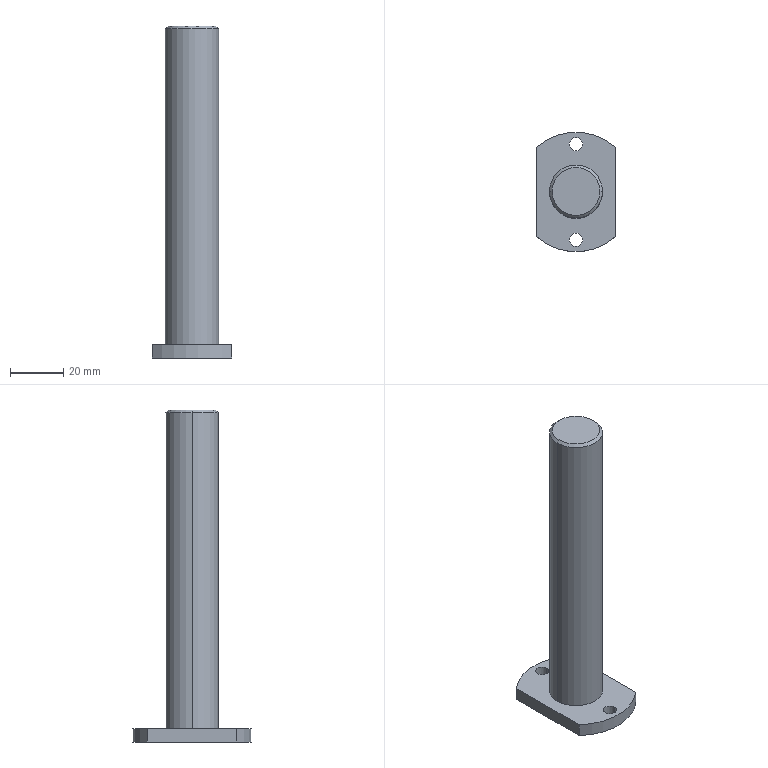Part | STEP file | Locking_pinV11 | 1 solid | 15 faces | box 30 x 45 x 125 mm | volume 43682 mm3 | cylinder 8 | plane 5 | cone 2 | commonest cylinder face diameters 5 x4 20 x2 45 x2
STEP:
#1=CARTESIAN_POINT('',(0.,0.,0.));
#2=DIRECTION('',(0.,0.,1.));
#3=DIRECTION('',(1.,0.,0.));
#4=AXIS2_PLACEMENT_3D('',#1,#2,#3);
#5=CARTESIAN_POINT('',(-2.5,18.,0.));
#6=VERTEX_POINT('',#5);
#7=CARTESIAN_POINT('',(-2.5,18.,-5.));
#8=VERTEX_POINT('',#7);
#9=CARTESIAN_POINT('',(-2.5,18.,-5.));
#10=DIRECTION('',(0.,0.,-1.));
#11=VECTOR('',#10,1.);
#12=LINE('',#9,#11);
#13=CARTESIAN_POINT('',(0.,18.,-5.));
#14=DIRECTION('',(0.,0.,-1.));
#15=DIRECTION('',(-1.,0.,0.));
#16=AXIS2_PLACEMENT_3D('',#13,#14,#15);
#17=CYLINDRICAL_SURFACE('',#16,2.5);
#18=CARTESIAN_POINT('',(6.283,0.));
#19=DIRECTION('',(0.,1.));
#20=VECTOR('',#19,1.);
#21=LINE('',#18,#20);
#22=(GEOMETRIC_REPRESENTATION_CONTEXT(2)PARAMETRIC_REPRESENTATION_CONTEXT()REPRESENTATION_CONTEXT('',''));
#23=DEFINITIONAL_REPRESENTATION('',(#21),#22);
#24=PCURVE('',#17,#23);
#25=CARTESIAN_POINT('',(0.,18.,-5.));
#26=DIRECTION('',(0.,0.,-1.));
#27=DIRECTION('',(-1.,0.,0.));
#28=AXIS2_PLACEMENT_3D('',#25,#26,#27);
#29=CYLINDRICAL_SURFACE('',#28,2.5);
#30=CARTESIAN_POINT('',(0.,0.));
#31=DIRECTION('',(0.,1.));
#32=VECTOR('',#31,1.);
#33=LINE('',#30,#32);
#34=(GEOMETRIC_REPRESENTATION_CONTEXT(2)PARAMETRIC_REPRESENTATION_CONTEXT()REPRESENTATION_CONTEXT('',''));
#35=DEFINITIONAL_REPRESENTATION('',(#33),#34);
#36=PCURVE('',#29,#35);
#37=SURFACE_CURVE('',#12,(#24,#36),.PCURVE_S1.);
#38=EDGE_CURVE('',#6,#8,#37,.T.);
#39=ORIENTED_EDGE('',*,*,#38,.T.);
#40=CARTESIAN_POINT('',(2.5,18.,-5.));
#41=VERTEX_POINT('',#40);
#42=CARTESIAN_POINT('',(0.,18.,-5.));
#43=DIRECTION('',(0.,0.,-1.));
#44=DIRECTION('',(-1.,0.,0.));
#45=AXIS2_PLACEMENT_3D('',#42,#43,#44);
#46=CIRCLE('',#45,2.5);
#47=CARTESIAN_POINT('',(0.,0.));
#48=DIRECTION('',(1.,0.));
#49=VECTOR('',#48,1.);
#50=LINE('',#47,#49);
#51=(GEOMETRIC_REPRESENTATION_CONTEXT(2)PARAMETRIC_REPRESENTATION_CONTEXT()REPRESENTATION_CONTEXT('',''));
#52=DEFINITIONAL_REPRESENTATION('',(#50),#51);
#53=PCURVE('',#17,#52);
#54=CARTESIAN_POINT('',(0.,0.,-5.));
#55=DIRECTION('',(0.,0.,-1.));
#56=DIRECTION('',(-1.,0.,0.));
#57=AXIS2_PLACEMENT_3D('',#54,#55,#56);
#58=PLANE('',#57);
#59=CARTESIAN_POINT('',(0.,18.));
#60=DIRECTION('',(1.,0.));
#61=AXIS2_PLACEMENT_2D('',#59,#60);
#62=CIRCLE('',#61,2.5);
#63=(GEOMETRIC_REPRESENTATION_CONTEXT(2)PARAMETRIC_REPRESENTATION_CONTEXT()REPRESENTATION_CONTEXT('',''));
#64=DEFINITIONAL_REPRESENTATION('',(#62),#63);
#65=PCURVE('',#58,#64);
#66=SURFACE_CURVE('',#46,(#53,#65),.PCURVE_S1.);
#67=EDGE_CURVE('',#41,#8,#66,.T.);
#68=ORIENTED_EDGE('',*,*,#67,.F.);
#69=CARTESIAN_POINT('',(2.5,18.,0.));
#70=VERTEX_POINT('',#69);
#71=CARTESIAN_POINT('',(2.5,18.,-5.));
#72=DIRECTION('',(0.,0.,-1.));
#73=VECTOR('',#72,1.);
#74=LINE('',#71,#73);
#75=CARTESIAN_POINT('',(3.142,0.));
#76=DIRECTION('',(0.,1.));
#77=VECTOR('',#76,1.);
#78=LINE('',#75,#77);
#79=(GEOMETRIC_REPRESENTATION_CONTEXT(2)PARAMETRIC_REPRESENTATION_CONTEXT()REPRESENTATION_CONTEXT('',''));
#80=DEFINITIONAL_REPRESENTATION('',(#78),#79);
#81=PCURVE('',#17,#80);
#82=CARTESIAN_POINT('',(3.142,0.));
#83=DIRECTION('',(0.,1.));
#84=VECTOR('',#83,1.);
#85=LINE('',#82,#84);
#86=(GEOMETRIC_REPRESENTATION_CONTEXT(2)PARAMETRIC_REPRESENTATION_CONTEXT()REPRESENTATION_CONTEXT('',''));
#87=DEFINITIONAL_REPRESENTATION('',(#85),#86);
#88=PCURVE('',#29,#87);
#89=SURFACE_CURVE('',#74,(#81,#88),.PCURVE_S1.);
#90=EDGE_CURVE('',#70,#41,#89,.T.);
#91=ORIENTED_EDGE('',*,*,#90,.F.);
#92=CARTESIAN_POINT('',(0.,18.,0.));
#93=DIRECTION('',(0.,0.,-1.));
#94=DIRECTION('',(-1.,0.,0.));
#95=AXIS2_PLACEMENT_3D('',#92,#93,#94);
#96=CIRCLE('',#95,2.5);
#97=CARTESIAN_POINT('',(0.,-5.));
#98=DIRECTION('',(1.,0.));
#99=VECTOR('',#98,1.);
#100=LINE('',#97,#99);
#101=(GEOMETRIC_REPRESENTATION_CONTEXT(2)PARAMETRIC_REPRESENTATION_CONTEXT()REPRESENTATION_CONTEXT('',''));
#102=DEFINITIONAL_REPRESENTATION('',(#100),#101);
#103=PCURVE('',#17,#102);
#104=CARTESIAN_POINT('',(0.,0.,0.));
#105=DIRECTION('',(0.,0.,-1.));
#106=DIRECTION('',(-1.,0.,0.));
#107=AXIS2_PLACEMENT_3D('',#104,#105,#106);
#108=PLANE('',#107);
#109=CARTESIAN_POINT('',(0.,18.));
#110=DIRECTION('',(1.,0.));
#111=AXIS2_PLACEMENT_2D('',#109,#110);
#112=CIRCLE('',#111,2.5);
#113=(GEOMETRIC_REPRESENTATION_CONTEXT(2)PARAMETRIC_REPRESENTATION_CONTEXT()REPRESENTATION_CONTEXT('',''));
#114=DEFINITIONAL_REPRESENTATION('',(#112),#113);
#115=PCURVE('',#108,#114);
#116=SURFACE_CURVE('',#96,(#103,#115),.PCURVE_S1.);
#117=EDGE_CURVE('',#70,#6,#116,.T.);
#118=ORIENTED_EDGE('',*,*,#117,.T.);
#119=EDGE_LOOP('',(#39,#68,#91,#118));
#120=FACE_BOUND('',#119,.F.);
#121=ADVANCED_FACE('',(#120),#17,.F.);
#122=CARTESIAN_POINT('',(-2.5,-18.,0.));
#123=VERTEX_POINT('',#122);
#124=CARTESIAN_POINT('',(-2.5,-18.,-5.));
#125=VERTEX_POINT('',#124);
#126=CARTESIAN_POINT('',(-2.5,-18.,-5.));
#127=DIRECTION('',(0.,0.,-1.));
#128=VECTOR('',#127,1.);
#129=LINE('',#126,#128);
#130=CARTESIAN_POINT('',(0.,-18.,-5.));
#131=DIRECTION('',(0.,0.,-1.));
#132=DIRECTION('',(-1.,0.,0.));
#133=AXIS2_PLACEMENT_3D('',#130,#131,#132);
#134=CYLINDRICAL_SURFACE('',#133,2.5);
#135=CARTESIAN_POINT('',(6.283,0.));
#136=DIRECTION('',(0.,1.));
#137=VECTOR('',#136,1.);
#138=LINE('',#135,#137);
#139=(GEOMETRIC_REPRESENTATION_CONTEXT(2)PARAMETRIC_REPRESENTATION_CONTEXT()REPRESENTATION_CONTEXT('',''));
#140=DEFINITIONAL_REPRESENTATION('',(#138),#139);
#141=PCURVE('',#134,#140);
#142=CARTESIAN_POINT('',(0.,-18.,-5.));
#143=DIRECTION('',(0.,0.,-1.));
#144=DIRECTION('',(-1.,0.,0.));
#145=AXIS2_PLACEMENT_3D('',#142,#143,#144);
#146=CYLINDRICAL_SURFACE('',#145,2.5);
#147=CARTESIAN_POINT('',(0.,0.));
#148=DIRECTION('',(0.,1.));
#149=VECTOR('',#148,1.);
#150=LINE('',#147,#149);
#151=(GEOMETRIC_REPRESENTATION_CONTEXT(2)PARAMETRIC_REPRESENTATION_CONTEXT()REPRESENTATION_CONTEXT('',''));
#152=DEFINITIONAL_REPRESENTATION('',(#150),#151);
#153=PCURVE('',#146,#152);
#154=SURFACE_CURVE('',#129,(#141,#153),.PCURVE_S1.);
#155=EDGE_CURVE('',#123,#125,#154,.T.);
#156=ORIENTED_EDGE('',*,*,#155,.T.);
#157=CARTESIAN_POINT('',(2.5,-18.,-5.));
#158=VERTEX_POINT('',#157);
#159=CARTESIAN_POINT('',(0.,-18.,-5.));
#160=DIRECTION('',(0.,0.,-1.));
#161=DIRECTION('',(-1.,0.,0.));
#162=AXIS2_PLACEMENT_3D('',#159,#160,#161);
#163=CIRCLE('',#162,2.5);
#164=CARTESIAN_POINT('',(0.,0.));
#165=DIRECTION('',(1.,0.));
#166=VECTOR('',#165,1.);
#167=LINE('',#164,#166);
#168=(GEOMETRIC_REPRESENTATION_CONTEXT(2)PARAMETRIC_REPRESENTATION_CONTEXT()REPRESENTATION_CONTEXT('',''));
#169=DEFINITIONAL_REPRESENTATION('',(#167),#168);
#170=PCURVE('',#134,#169);
#171=CARTESIAN_POINT('',(0.,-18.));
#172=DIRECTION('',(1.,0.));
#173=AXIS2_PLACEMENT_2D('',#171,#172);
#174=CIRCLE('',#173,2.5);
#175=(GEOMETRIC_REPRESENTATION_CONTEXT(2)PARAMETRIC_REPRESENTATION_CONTEXT()REPRESENTATION_CONTEXT('',''));
#176=DEFINITIONAL_REPRESENTATION('',(#174),#175);
#177=PCURVE('',#58,#176);
#178=SURFACE_CURVE('',#163,(#170,#177),.PCURVE_S1.);
#179=EDGE_CURVE('',#158,#125,#178,.T.);
#180=ORIENTED_EDGE('',*,*,#179,.F.);
#181=CARTESIAN_POINT('',(2.5,-18.,0.));
#182=VERTEX_POINT('',#181);
#183=CARTESIAN_POINT('',(2.5,-18.,-5.));
#184=DIRECTION('',(0.,0.,-1.));
#185=VECTOR('',#184,1.);
#186=LINE('',#183,#185);
#187=CARTESIAN_POINT('',(3.142,0.));
#188=DIRECTION('',(0.,1.));
#189=VECTOR('',#188,1.);
#190=LINE('',#187,#189);
#191=(GEOMETRIC_REPRESENTATION_CONTEXT(2)PARAMETRIC_REPRESENTATION_CONTEXT()REPRESENTATION_CONTEXT('',''));
#192=DEFINITIONAL_REPRESENTATION('',(#190),#191);
#193=PCURVE('',#134,#192);
#194=CARTESIAN_POINT('',(3.142,0.));
#195=DIRECTION('',(0.,1.));
#196=VECTOR('',#195,1.);
#197=LINE('',#194,#196);
#198=(GEOMETRIC_REPRESENTATION_CONTEXT(2)PARAMETRIC_REPRESENTATION_CONTEXT()REPRESENTATION_CONTEXT('',''));
#199=DEFINITIONAL_REPRESENTATION('',(#197),#198);
#200=PCURVE('',#146,#199);
#201=SURFACE_CURVE('',#186,(#193,#200),.PCURVE_S1.);
#202=EDGE_CURVE('',#182,#158,#201,.T.);
#203=ORIENTED_EDGE('',*,*,#202,.F.);
#204=CARTESIAN_POINT('',(0.,-18.,0.));
#205=DIRECTION('',(0.,0.,-1.));
#206=DIRECTION('',(-1.,0.,0.));
#207=AXIS2_PLACEMENT_3D('',#204,#205,#206);
#208=CIRCLE('',#207,2.5);
#209=CARTESIAN_POINT('',(0.,-5.));
#210=DIRECTION('',(1.,0.));
#211=VECTOR('',#210,1.);
#212=LINE('',#209,#211);
#213=(GEOMETRIC_REPRESENTATION_CONTEXT(2)PARAMETRIC_REPRESENTATION_CONTEXT()REPRESENTATION_CONTEXT('',''));
#214=DEFINITIONAL_REPRESENTATION('',(#212),#213);
#215=PCURVE('',#134,#214);
#216=CARTESIAN_POINT('',(0.,-18.));
#217=DIRECTION('',(1.,0.));
#218=AXIS2_PLACEMENT_2D('',#216,#217);
#219=CIRCLE('',#218,2.5);
#220=(GEOMETRIC_REPRESENTATION_CONTEXT(2)PARAMETRIC_REPRESENTATION_CONTEXT()REPRESENTATION_CONTEXT('',''));
#221=DEFINITIONAL_REPRESENTATION('',(#219),#220);
#222=PCURVE('',#108,#221);
#223=SURFACE_CURVE('',#208,(#215,#222),.PCURVE_S1.);
#224=EDGE_CURVE('',#182,#123,#223,.T.);
#225=ORIENTED_EDGE('',*,*,#224,.T.);
#226=EDGE_LOOP('',(#156,#180,#203,#225));
#227=FACE_BOUND('',#226,.F.);
#228=ADVANCED_FACE('',(#227),#134,.F.);
#229=CARTESIAN_POINT('',(9.,0.,120.));
#230=VERTEX_POINT('',#229);
#231=CARTESIAN_POINT('',(-9.,0.,120.));
#232=VERTEX_POINT('',#231);
#233=CARTESIAN_POINT('',(0.,0.,120.));
#234=DIRECTION('',(0.,0.,1.));
#235=DIRECTION('',(1.,0.,0.));
#236=AXIS2_PLACEMENT_3D('',#233,#234,#235);
#237=CIRCLE('',#236,9.);
#238=CARTESIAN_POINT('',(0.,0.,120.));
#239=DIRECTION('',(0.,0.,-1.));
#240=DIRECTION('',(-1.,0.,0.));
#241=AXIS2_PLACEMENT_3D('',#238,#239,#240);
#242=CONICAL_SURFACE('',#241,9.,0.7854);
#243=CARTESIAN_POINT('',(3.142,0.));
#244=DIRECTION('',(-1.,0.));
#245=VECTOR('',#244,1.);
#246=LINE('',#243,#245);
#247=(GEOMETRIC_REPRESENTATION_CONTEXT(2)PARAMETRIC_REPRESENTATION_CONTEXT()REPRESENTATION_CONTEXT('',''));
#248=DEFINITIONAL_REPRESENTATION('',(#246),#247);
#249=PCURVE('',#242,#248);
#250=CARTESIAN_POINT('',(0.,0.,120.));
#251=DIRECTION('',(0.,0.,1.));
#252=DIRECTION('',(1.,0.,0.));
#253=AXIS2_PLACEMENT_3D('',#250,#251,#252);
#254=PLANE('',#253);
#255=CARTESIAN_POINT('',(0.,0.));
#256=DIRECTION('',(1.,0.));
#257=AXIS2_PLACEMENT_2D('',#255,#256);
#258=CIRCLE('',#257,9.);
#259=(GEOMETRIC_REPRESENTATION_CONTEXT(2)PARAMETRIC_REPRESENTATION_CONTEXT()REPRESENTATION_CONTEXT('',''));
#260=DEFINITIONAL_REPRESENTATION('',(#258),#259);
#261=PCURVE('',#254,#260);
#262=SURFACE_CURVE('',#237,(#249,#261),.PCURVE_S1.);
#263=EDGE_CURVE('',#230,#232,#262,.T.);
#264=ORIENTED_EDGE('',*,*,#263,.F.);
#265=CARTESIAN_POINT('',(10.,0.,119.));
#266=VERTEX_POINT('',#265);
#267=CARTESIAN_POINT('',(9.,0.,120.));
#268=DIRECTION('',(0.7071,0.,-0.7071));
#269=VECTOR('',#268,1.);
#270=LINE('',#267,#269);
#271=CARTESIAN_POINT('',(3.142,0.));
#272=DIRECTION('',(0.,1.));
#273=VECTOR('',#272,1.);
#274=LINE('',#271,#273);
#275=(GEOMETRIC_REPRESENTATION_CONTEXT(2)PARAMETRIC_REPRESENTATION_CONTEXT()REPRESENTATION_CONTEXT('',''));
#276=DEFINITIONAL_REPRESENTATION('',(#274),#275);
#277=PCURVE('',#242,#276);
#278=CARTESIAN_POINT('',(0.,0.,120.));
#279=DIRECTION('',(0.,0.,-1.));
#280=DIRECTION('',(-1.,0.,0.));
#281=AXIS2_PLACEMENT_3D('',#278,#279,#280);
#282=CONICAL_SURFACE('',#281,9.,0.7854);
#283=CARTESIAN_POINT('',(3.142,0.));
#284=DIRECTION('',(0.,1.));
#285=VECTOR('',#284,1.);
#286=LINE('',#283,#285);
#287=(GEOMETRIC_REPRESENTATION_CONTEXT(2)PARAMETRIC_REPRESENTATION_CONTEXT()REPRESENTATION_CONTEXT('',''));
#288=DEFINITIONAL_REPRESENTATION('',(#286),#287);
#289=PCURVE('',#282,#288);
#290=SURFACE_CURVE('',#270,(#277,#289),.PCURVE_S1.);
#291=EDGE_CURVE('',#230,#266,#290,.T.);
#292=ORIENTED_EDGE('',*,*,#291,.T.);
#293=CARTESIAN_POINT('',(-10.,0.,119.));
#294=VERTEX_POINT('',#293);
#295=CARTESIAN_POINT('',(0.,0.,119.));
#296=DIRECTION('',(0.,0.,-1.));
#297=DIRECTION('',(1.,0.,0.));
#298=AXIS2_PLACEMENT_3D('',#295,#296,#297);
#299=CIRCLE('',#298,10.);
#300=CARTESIAN_POINT('',(-3.142,1.));
#301=DIRECTION('',(1.,0.));
#302=VECTOR('',#301,1.);
#303=LINE('',#300,#302);
#304=(GEOMETRIC_REPRESENTATION_CONTEXT(2)PARAMETRIC_REPRESENTATION_CONTEXT()REPRESENTATION_CONTEXT('',''));
#305=DEFINITIONAL_REPRESENTATION('',(#303),#304);
#306=PCURVE('',#242,#305);
#307=CARTESIAN_POINT('',(0.,0.,120.));
#308=DIRECTION('',(0.,0.,-1.));
#309=DIRECTION('',(-1.,0.,0.));
#310=AXIS2_PLACEMENT_3D('',#307,#308,#309);
#311=CYLINDRICAL_SURFACE('',#310,10.);
#312=CARTESIAN_POINT('',(-3.142,1.));
#313=DIRECTION('',(1.,0.));
#314=VECTOR('',#313,1.);
#315=LINE('',#312,#314);
#316=(GEOMETRIC_REPRESENTATION_CONTEXT(2)PARAMETRIC_REPRESENTATION_CONTEXT()REPRESENTATION_CONTEXT('',''));
#317=DEFINITIONAL_REPRESENTATION('',(#315),#316);
#318=PCURVE('',#311,#317);
#319=SURFACE_CURVE('',#299,(#306,#318),.PCURVE_S1.);
#320=EDGE_CURVE('',#294,#266,#319,.T.);
#321=ORIENTED_EDGE('',*,*,#320,.F.);
#322=CARTESIAN_POINT('',(-9.,0.,120.));
#323=DIRECTION('',(-0.7071,0.,-0.7071));
#324=VECTOR('',#323,1.);
#325=LINE('',#322,#324);
#326=CARTESIAN_POINT('',(0.,0.));
#327=DIRECTION('',(0.,1.));
#328=VECTOR('',#327,1.);
#329=LINE('',#326,#328);
#330=(GEOMETRIC_REPRESENTATION_CONTEXT(2)PARAMETRIC_REPRESENTATION_CONTEXT()REPRESENTATION_CONTEXT('',''));
#331=DEFINITIONAL_REPRESENTATION('',(#329),#330);
#332=PCURVE('',#242,#331);
#333=CARTESIAN_POINT('',(6.283,0.));
#334=DIRECTION('',(0.,1.));
#335=VECTOR('',#334,1.);
#336=LINE('',#333,#335);
#337=(GEOMETRIC_REPRESENTATION_CONTEXT(2)PARAMETRIC_REPRESENTATION_CONTEXT()REPRESENTATION_CONTEXT('',''));
#338=DEFINITIONAL_REPRESENTATION('',(#336),#337);
#339=PCURVE('',#282,#338);
#340=SURFACE_CURVE('',#325,(#332,#339),.PCURVE_S1.);
#341=EDGE_CURVE('',#232,#294,#340,.T.);
#342=ORIENTED_EDGE('',*,*,#341,.F.);
#343=EDGE_LOOP('',(#264,#292,#321,#342));
#344=FACE_BOUND('',#343,.T.);
#345=ADVANCED_FACE('',(#344),#242,.T.);
#346=ORIENTED_EDGE('',*,*,#320,.T.);
#347=CARTESIAN_POINT('',(10.,0.,0.));
#348=VERTEX_POINT('',#347);
#349=CARTESIAN_POINT('',(10.,0.,120.));
#350=DIRECTION('',(0.,0.,-1.));
#351=VECTOR('',#350,1.);
#352=LINE('',#349,#351);
#353=CARTESIAN_POINT('',(3.142,0.));
#354=DIRECTION('',(0.,1.));
#355=VECTOR('',#354,1.);
#356=LINE('',#353,#355);
#357=(GEOMETRIC_REPRESENTATION_CONTEXT(2)PARAMETRIC_REPRESENTATION_CONTEXT()REPRESENTATION_CONTEXT('',''));
#358=DEFINITIONAL_REPRESENTATION('',(#356),#357);
#359=PCURVE('',#311,#358);
#360=CARTESIAN_POINT('',(0.,0.,120.));
#361=DIRECTION('',(0.,0.,-1.));
#362=DIRECTION('',(-1.,0.,0.));
#363=AXIS2_PLACEMENT_3D('',#360,#361,#362);
#364=CYLINDRICAL_SURFACE('',#363,10.);
#365=CARTESIAN_POINT('',(3.142,0.));
#366=DIRECTION('',(0.,1.));
#367=VECTOR('',#366,1.);
#368=LINE('',#365,#367);
#369=(GEOMETRIC_REPRESENTATION_CONTEXT(2)PARAMETRIC_REPRESENTATION_CONTEXT()REPRESENTATION_CONTEXT('',''));
#370=DEFINITIONAL_REPRESENTATION('',(#368),#369);
#371=PCURVE('',#364,#370);
#372=SURFACE_CURVE('',#352,(#359,#371),.PCURVE_S1.);
#373=EDGE_CURVE('',#266,#348,#372,.T.);
#374=ORIENTED_EDGE('',*,*,#373,.T.);
#375=CARTESIAN_POINT('',(-10.,0.,0.));
#376=VERTEX_POINT('',#375);
#377=CARTESIAN_POINT('',(0.,0.,0.));
#378=DIRECTION('',(0.,0.,1.));
#379=DIRECTION('',(1.,0.,0.));
#380=AXIS2_PLACEMENT_3D('',#377,#378,#379);
#381=CIRCLE('',#380,10.);
#382=CARTESIAN_POINT('',(3.142,120.));
#383=DIRECTION('',(-1.,0.));
#384=VECTOR('',#383,1.);
#385=LINE('',#382,#384);
#386=(GEOMETRIC_REPRESENTATION_CONTEXT(2)PARAMETRIC_REPRESENTATION_CONTEXT()REPRESENTATION_CONTEXT('',''));
#387=DEFINITIONAL_REPRESENTATION('',(#385),#386);
#388=PCURVE('',#311,#387);
#389=CARTESIAN_POINT('',(-10.,0.));
#390=CARTESIAN_POINT('',(-10.,17.321));
#391=CARTESIAN_POINT('',(5.,8.66));
#392=CARTESIAN_POINT('',(20.,0.));
#393=CARTESIAN_POINT('',(5.,-8.66));
#394=CARTESIAN_POINT('',(-10.,-17.321));
#395=CARTESIAN_POINT('',(-10.,0.));
#396=(BOUNDED_CURVE()B_SPLINE_CURVE(2,(#389,#390,#391,#392,#393,#394,#395),.UNSPECIFIED.,.T.,.F.)B_SPLINE_CURVE_WITH_KNOTS((1,2,2,2,2,1),(-2.094,0.,2.094,4.189,6.283,8.378),.UNSPECIFIED.)CURVE()GEOMETRIC_REPRESENTATION_ITEM()RATIONAL_B_SPLINE_CURVE((1.,0.5,1.,0.5,1.,0.5,1.))REPRESENTATION_ITEM(''));
#397=(GEOMETRIC_REPRESENTATION_CONTEXT(2)PARAMETRIC_REPRESENTATION_CONTEXT()REPRESENTATION_CONTEXT('',''));
#398=DEFINITIONAL_REPRESENTATION('',(#396),#397);
#399=PCURVE('',#108,#398);
#400=SURFACE_CURVE('',#381,(#388,#399),.PCURVE_S1.);
#401=EDGE_CURVE('',#348,#376,#400,.T.);
#402=ORIENTED_EDGE('',*,*,#401,.T.);
#403=CARTESIAN_POINT('',(-10.,0.,120.));
#404=DIRECTION('',(0.,0.,-1.));
#405=VECTOR('',#404,1.);
#406=LINE('',#403,#405);
#407=CARTESIAN_POINT('',(0.,0.));
#408=DIRECTION('',(0.,1.));
#409=VECTOR('',#408,1.);
#410=LINE('',#407,#409);
#411=(GEOMETRIC_REPRESENTATION_CONTEXT(2)PARAMETRIC_REPRESENTATION_CONTEXT()REPRESENTATION_CONTEXT('',''));
#412=DEFINITIONAL_REPRESENTATION('',(#410),#411);
#413=PCURVE('',#311,#412);
#414=CARTESIAN_POINT('',(6.283,0.));
#415=DIRECTION('',(0.,1.));
#416=VECTOR('',#415,1.);
#417=LINE('',#414,#416);
#418=(GEOMETRIC_REPRESENTATION_CONTEXT(2)PARAMETRIC_REPRESENTATION_CONTEXT()REPRESENTATION_CONTEXT('',''));
#419=DEFINITIONAL_REPRESENTATION('',(#417),#418);
#420=PCURVE('',#364,#419);
#421=SURFACE_CURVE('',#406,(#413,#420),.PCURVE_S1.);
#422=EDGE_CURVE('',#294,#376,#421,.T.);
#423=ORIENTED_EDGE('',*,*,#422,.F.);
#424=EDGE_LOOP('',(#346,#374,#402,#423));
#425=FACE_BOUND('',#424,.T.);
#426=ADVANCED_FACE('',(#425),#311,.T.);
#427=ORIENTED_EDGE('',*,*,#373,.F.);
#428=CARTESIAN_POINT('',(0.,0.,119.));
#429=DIRECTION('',(0.,0.,-1.));
#430=DIRECTION('',(1.,0.,0.));
#431=AXIS2_PLACEMENT_3D('',#428,#429,#430);
#432=CIRCLE('',#431,10.);
#433=CARTESIAN_POINT('',(3.142,1.));
#434=DIRECTION('',(1.,0.));
#435=VECTOR('',#434,1.);
#436=LINE('',#433,#435);
#437=(GEOMETRIC_REPRESENTATION_CONTEXT(2)PARAMETRIC_REPRESENTATION_CONTEXT()REPRESENTATION_CONTEXT('',''));
#438=DEFINITIONAL_REPRESENTATION('',(#436),#437);
#439=PCURVE('',#364,#438);
#440=CARTESIAN_POINT('',(3.142,1.));
#441=DIRECTION('',(1.,0.));
#442=VECTOR('',#441,1.);
#443=LINE('',#440,#442);
#444=(GEOMETRIC_REPRESENTATION_CONTEXT(2)PARAMETRIC_REPRESENTATION_CONTEXT()REPRESENTATION_CONTEXT('',''));
#445=DEFINITIONAL_REPRESENTATION('',(#443),#444);
#446=PCURVE('',#282,#445);
#447=SURFACE_CURVE('',#432,(#439,#446),.PCURVE_S1.);
#448=EDGE_CURVE('',#266,#294,#447,.T.);
#449=ORIENTED_EDGE('',*,*,#448,.T.);
#450=ORIENTED_EDGE('',*,*,#422,.T.);
#451=CARTESIAN_POINT('',(0.,0.,0.));
#452=DIRECTION('',(0.,0.,1.));
#453=DIRECTION('',(1.,0.,0.));
#454=AXIS2_PLACEMENT_3D('',#451,#452,#453);
#455=CIRCLE('',#454,10.);
#456=CARTESIAN_POINT('',(9.425,120.));
#457=DIRECTION('',(-1.,0.));
#458=VECTOR('',#457,1.);
#459=LINE('',#456,#458);
#460=(GEOMETRIC_REPRESENTATION_CONTEXT(2)PARAMETRIC_REPRESENTATION_CONTEXT()REPRESENTATION_CONTEXT('',''));
#461=DEFINITIONAL_REPRESENTATION('',(#459),#460);
#462=PCURVE('',#364,#461);
#463=CARTESIAN_POINT('',(-10.,0.));
#464=CARTESIAN_POINT('',(-10.,17.321));
#465=CARTESIAN_POINT('',(5.,8.66));
#466=CARTESIAN_POINT('',(20.,0.));
#467=CARTESIAN_POINT('',(5.,-8.66));
#468=CARTESIAN_POINT('',(-10.,-17.321));
#469=CARTESIAN_POINT('',(-10.,0.));
#470=(BOUNDED_CURVE()B_SPLINE_CURVE(2,(#463,#464,#465,#466,#467,#468,#469),.UNSPECIFIED.,.T.,.F.)B_SPLINE_CURVE_WITH_KNOTS((1,2,2,2,2,1),(-2.094,0.,2.094,4.189,6.283,8.378),.UNSPECIFIED.)CURVE()GEOMETRIC_REPRESENTATION_ITEM()RATIONAL_B_SPLINE_CURVE((1.,0.5,1.,0.5,1.,0.5,1.))REPRESENTATION_ITEM(''));
#471=(GEOMETRIC_REPRESENTATION_CONTEXT(2)PARAMETRIC_REPRESENTATION_CONTEXT()REPRESENTATION_CONTEXT('',''));
#472=DEFINITIONAL_REPRESENTATION('',(#470),#471);
#473=PCURVE('',#108,#472);
#474=SURFACE_CURVE('',#455,(#462,#473),.PCURVE_S1.);
#475=EDGE_CURVE('',#376,#348,#474,.T.);
#476=ORIENTED_EDGE('',*,*,#475,.T.);
#477=EDGE_LOOP('',(#427,#449,#450,#476));
#478=FACE_BOUND('',#477,.T.);
#479=ADVANCED_FACE('',(#478),#364,.T.);
#480=CARTESIAN_POINT('',(0.,0.,120.));
#481=DIRECTION('',(0.,0.,1.));
#482=DIRECTION('',(1.,0.,0.));
#483=AXIS2_PLACEMENT_3D('',#480,#481,#482);
#484=CIRCLE('',#483,9.);
#485=CARTESIAN_POINT('',(0.,0.));
#486=DIRECTION('',(1.,0.));
#487=AXIS2_PLACEMENT_2D('',#485,#486);
#488=CIRCLE('',#487,9.);
#489=(GEOMETRIC_REPRESENTATION_CONTEXT(2)PARAMETRIC_REPRESENTATION_CONTEXT()REPRESENTATION_CONTEXT('',''));
#490=DEFINITIONAL_REPRESENTATION('',(#488),#489);
#491=PCURVE('',#254,#490);
#492=CARTESIAN_POINT('',(9.425,0.));
#493=DIRECTION('',(-1.,0.));
#494=VECTOR('',#493,1.);
#495=LINE('',#492,#494);
#496=(GEOMETRIC_REPRESENTATION_CONTEXT(2)PARAMETRIC_REPRESENTATION_CONTEXT()REPRESENTATION_CONTEXT('',''));
#497=DEFINITIONAL_REPRESENTATION('',(#495),#496);
#498=PCURVE('',#282,#497);
#499=SURFACE_CURVE('',#484,(#491,#498),.PCURVE_S1.);
#500=EDGE_CURVE('',#232,#230,#499,.T.);
#501=ORIENTED_EDGE('',*,*,#500,.T.);
#502=ORIENTED_EDGE('',*,*,#263,.T.);
#503=EDGE_LOOP('',(#501,#502));
#504=FACE_BOUND('',#503,.T.);
#505=ADVANCED_FACE('',(#504),#254,.T.);
#506=ORIENTED_EDGE('',*,*,#291,.F.);
#507=ORIENTED_EDGE('',*,*,#500,.F.);
#508=ORIENTED_EDGE('',*,*,#341,.T.);
#509=ORIENTED_EDGE('',*,*,#448,.F.);
#510=EDGE_LOOP('',(#506,#507,#508,#509));
#511=FACE_BOUND('',#510,.T.);
#512=ADVANCED_FACE('',(#511),#282,.T.);
#513=CARTESIAN_POINT('',(15.,-16.771,0.));
#514=VERTEX_POINT('',#513);
#515=CARTESIAN_POINT('',(-15.,-16.771,0.));
#516=VERTEX_POINT('',#515);
#517=CARTESIAN_POINT('',(0.,0.,0.));
#518=DIRECTION('',(0.,0.,-1.));
#519=DIRECTION('',(-1.,0.,0.));
#520=AXIS2_PLACEMENT_3D('',#517,#518,#519);
#521=CIRCLE('',#520,22.5);
#522=CARTESIAN_POINT('',(0.,0.,-5.));
#523=DIRECTION('',(0.,0.,1.));
#524=DIRECTION('',(1.,0.,0.));
#525=AXIS2_PLACEMENT_3D('',#522,#523,#524);
#526=CYLINDRICAL_SURFACE('',#525,22.5);
#527=CARTESIAN_POINT('',(9.425,5.));
#528=DIRECTION('',(-1.,0.));
#529=VECTOR('',#528,1.);
#530=LINE('',#527,#529);
#531=(GEOMETRIC_REPRESENTATION_CONTEXT(2)PARAMETRIC_REPRESENTATION_CONTEXT()REPRESENTATION_CONTEXT('',''));
#532=DEFINITIONAL_REPRESENTATION('',(#530),#531);
#533=PCURVE('',#526,#532);
#534=CARTESIAN_POINT('',(0.,0.));
#535=DIRECTION('',(1.,0.));
#536=AXIS2_PLACEMENT_2D('',#534,#535);
#537=CIRCLE('',#536,22.5);
#538=(GEOMETRIC_REPRESENTATION_CONTEXT(2)PARAMETRIC_REPRESENTATION_CONTEXT()REPRESENTATION_CONTEXT('',''));
#539=DEFINITIONAL_REPRESENTATION('',(#537),#538);
#540=PCURVE('',#108,#539);
#541=SURFACE_CURVE('',#521,(#533,#540),.PCURVE_S1.);
#542=EDGE_CURVE('',#514,#516,#541,.T.);
#543=ORIENTED_EDGE('',*,*,#542,.T.);
#544=CARTESIAN_POINT('',(-15.,-16.771,-5.));
#545=VERTEX_POINT('',#544);
#546=CARTESIAN_POINT('',(-15.,-16.771,-5.));
#547=DIRECTION('',(0.,0.,1.));
#548=VECTOR('',#547,1.);
#549=LINE('',#546,#548);
#550=CARTESIAN_POINT('',(3.983,0.));
#551=DIRECTION('',(0.,1.));
#552=VECTOR('',#551,1.);
#553=LINE('',#550,#552);
#554=(GEOMETRIC_REPRESENTATION_CONTEXT(2)PARAMETRIC_REPRESENTATION_CONTEXT()REPRESENTATION_CONTEXT('',''));
#555=DEFINITIONAL_REPRESENTATION('',(#553),#554);
#556=PCURVE('',#526,#555);
#557=CARTESIAN_POINT('',(-15.,16.771,-5.));
#558=DIRECTION('',(1.,0.,0.));
#559=DIRECTION('',(0.,0.,-1.));
#560=AXIS2_PLACEMENT_3D('',#557,#558,#559);
#561=PLANE('',#560);
#562=CARTESIAN_POINT('',(0.,-33.541));
#563=DIRECTION('',(-1.,0.));
#564=VECTOR('',#563,1.);
#565=LINE('',#562,#564);
#566=(GEOMETRIC_REPRESENTATION_CONTEXT(2)PARAMETRIC_REPRESENTATION_CONTEXT()REPRESENTATION_CONTEXT('',''));
#567=DEFINITIONAL_REPRESENTATION('',(#565),#566);
#568=PCURVE('',#561,#567);
#569=SURFACE_CURVE('',#549,(#556,#568),.PCURVE_S1.);
#570=EDGE_CURVE('',#545,#516,#569,.T.);
#571=ORIENTED_EDGE('',*,*,#570,.F.);
#572=CARTESIAN_POINT('',(15.,-16.771,-5.));
#573=VERTEX_POINT('',#572);
#574=CARTESIAN_POINT('',(0.,0.,-5.));
#575=DIRECTION('',(0.,0.,-1.));
#576=DIRECTION('',(-1.,0.,0.));
#577=AXIS2_PLACEMENT_3D('',#574,#575,#576);
#578=CIRCLE('',#577,22.5);
#579=CARTESIAN_POINT('',(9.425,0.));
#580=DIRECTION('',(-1.,0.));
#581=VECTOR('',#580,1.);
#582=LINE('',#579,#581);
#583=(GEOMETRIC_REPRESENTATION_CONTEXT(2)PARAMETRIC_REPRESENTATION_CONTEXT()REPRESENTATION_CONTEXT('',''));
#584=DEFINITIONAL_REPRESENTATION('',(#582),#583);
#585=PCURVE('',#526,#584);
#586=CARTESIAN_POINT('',(0.,0.));
#587=DIRECTION('',(1.,0.));
#588=AXIS2_PLACEMENT_2D('',#586,#587);
#589=CIRCLE('',#588,22.5);
#590=(GEOMETRIC_REPRESENTATION_CONTEXT(2)PARAMETRIC_REPRESENTATION_CONTEXT()REPRESENTATION_CONTEXT('',''));
#591=DEFINITIONAL_REPRESENTATION('',(#589),#590);
#592=PCURVE('',#58,#591);
#593=SURFACE_CURVE('',#578,(#585,#592),.PCURVE_S1.);
#594=EDGE_CURVE('',#573,#545,#593,.T.);
#595=ORIENTED_EDGE('',*,*,#594,.F.);
#596=CARTESIAN_POINT('',(15.,-16.771,-5.));
#597=DIRECTION('',(0.,0.,1.));
#598=VECTOR('',#597,1.);
#599=LINE('',#596,#598);
#600=CARTESIAN_POINT('',(5.442,0.));
#601=DIRECTION('',(0.,1.));
#602=VECTOR('',#601,1.);
#603=LINE('',#600,#602);
#604=(GEOMETRIC_REPRESENTATION_CONTEXT(2)PARAMETRIC_REPRESENTATION_CONTEXT()REPRESENTATION_CONTEXT('',''));
#605=DEFINITIONAL_REPRESENTATION('',(#603),#604);
#606=PCURVE('',#526,#605);
#607=CARTESIAN_POINT('',(15.,16.771,-5.));
#608=DIRECTION('',(-1.,0.,0.));
#609=DIRECTION('',(0.,0.,1.));
#610=AXIS2_PLACEMENT_3D('',#607,#608,#609);
#611=PLANE('',#610);
#612=CARTESIAN_POINT('',(0.,-33.541));
#613=DIRECTION('',(1.,0.));
#614=VECTOR('',#613,1.);
#615=LINE('',#612,#614);
#616=(GEOMETRIC_REPRESENTATION_CONTEXT(2)PARAMETRIC_REPRESENTATION_CONTEXT()REPRESENTATION_CONTEXT('',''));
#617=DEFINITIONAL_REPRESENTATION('',(#615),#616);
#618=PCURVE('',#611,#617);
#619=SURFACE_CURVE('',#599,(#606,#618),.PCURVE_S1.);
#620=EDGE_CURVE('',#573,#514,#619,.T.);
#621=ORIENTED_EDGE('',*,*,#620,.T.);
#622=EDGE_LOOP('',(#543,#571,#595,#621));
#623=FACE_BOUND('',#622,.T.);
#624=ADVANCED_FACE('',(#623),#526,.T.);
#625=CARTESIAN_POINT('',(-15.,16.771,0.));
#626=VERTEX_POINT('',#625);
#627=CARTESIAN_POINT('',(-15.,16.771,0.));
#628=DIRECTION('',(0.,1.,0.));
#629=VECTOR('',#628,1.);
#630=LINE('',#627,#629);
#631=CARTESIAN_POINT('',(-5.,0.));
#632=DIRECTION('',(0.,1.));
#633=VECTOR('',#632,1.);
#634=LINE('',#631,#633);
#635=(GEOMETRIC_REPRESENTATION_CONTEXT(2)PARAMETRIC_REPRESENTATION_CONTEXT()REPRESENTATION_CONTEXT('',''));
#636=DEFINITIONAL_REPRESENTATION('',(#634),#635);
#637=PCURVE('',#561,#636);
#638=CARTESIAN_POINT('',(15.,16.771));
#639=DIRECTION('',(0.,1.));
#640=VECTOR('',#639,1.);
#641=LINE('',#638,#640);
#642=(GEOMETRIC_REPRESENTATION_CONTEXT(2)PARAMETRIC_REPRESENTATION_CONTEXT()REPRESENTATION_CONTEXT('',''));
#643=DEFINITIONAL_REPRESENTATION('',(#641),#642);
#644=PCURVE('',#108,#643);
#645=SURFACE_CURVE('',#630,(#637,#644),.PCURVE_S1.);
#646=EDGE_CURVE('',#516,#626,#645,.T.);
#647=ORIENTED_EDGE('',*,*,#646,.T.);
#648=CARTESIAN_POINT('',(-15.,16.771,-5.));
#649=VERTEX_POINT('',#648);
#650=CARTESIAN_POINT('',(-15.,16.771,-5.));
#651=DIRECTION('',(0.,0.,1.));
#652=VECTOR('',#651,1.);
#653=LINE('',#650,#652);
#654=CARTESIAN_POINT('',(0.,0.));
#655=DIRECTION('',(-1.,0.));
#656=VECTOR('',#655,1.);
#657=LINE('',#654,#656);
#658=(GEOMETRIC_REPRESENTATION_CONTEXT(2)PARAMETRIC_REPRESENTATION_CONTEXT()REPRESENTATION_CONTEXT('',''));
#659=DEFINITIONAL_REPRESENTATION('',(#657),#658);
#660=PCURVE('',#561,#659);
#661=CARTESIAN_POINT('',(0.,0.,-5.));
#662=DIRECTION('',(0.,0.,1.));
#663=DIRECTION('',(1.,0.,0.));
#664=AXIS2_PLACEMENT_3D('',#661,#662,#663);
#665=CYLINDRICAL_SURFACE('',#664,22.5);
#666=CARTESIAN_POINT('',(2.301,0.));
#667=DIRECTION('',(0.,1.));
#668=VECTOR('',#667,1.);
#669=LINE('',#666,#668);
#670=(GEOMETRIC_REPRESENTATION_CONTEXT(2)PARAMETRIC_REPRESENTATION_CONTEXT()REPRESENTATION_CONTEXT('',''));
#671=DEFINITIONAL_REPRESENTATION('',(#669),#670);
#672=PCURVE('',#665,#671);
#673=SURFACE_CURVE('',#653,(#660,#672),.PCURVE_S1.);
#674=EDGE_CURVE('',#649,#626,#673,.T.);
#675=ORIENTED_EDGE('',*,*,#674,.F.);
#676=CARTESIAN_POINT('',(-15.,16.771,-5.));
#677=DIRECTION('',(0.,1.,0.));
#678=VECTOR('',#677,1.);
#679=LINE('',#676,#678);
#680=CARTESIAN_POINT('',(0.,0.));
#681=DIRECTION('',(0.,1.));
#682=VECTOR('',#681,1.);
#683=LINE('',#680,#682);
#684=(GEOMETRIC_REPRESENTATION_CONTEXT(2)PARAMETRIC_REPRESENTATION_CONTEXT()REPRESENTATION_CONTEXT('',''));
#685=DEFINITIONAL_REPRESENTATION('',(#683),#684);
#686=PCURVE('',#561,#685);
#687=CARTESIAN_POINT('',(15.,16.771));
#688=DIRECTION('',(0.,1.));
#689=VECTOR('',#688,1.);
#690=LINE('',#687,#689);
#691=(GEOMETRIC_REPRESENTATION_CONTEXT(2)PARAMETRIC_REPRESENTATION_CONTEXT()REPRESENTATION_CONTEXT('',''));
#692=DEFINITIONAL_REPRESENTATION('',(#690),#691);
#693=PCURVE('',#58,#692);
#694=SURFACE_CURVE('',#679,(#686,#693),.PCURVE_S1.);
#695=EDGE_CURVE('',#545,#649,#694,.T.);
#696=ORIENTED_EDGE('',*,*,#695,.F.);
#697=ORIENTED_EDGE('',*,*,#570,.T.);
#698=EDGE_LOOP('',(#647,#675,#696,#697));
#699=FACE_BOUND('',#698,.T.);
#700=ADVANCED_FACE('',(#699),#561,.F.);
#701=CARTESIAN_POINT('',(15.,16.771,0.));
#702=VERTEX_POINT('',#701);
#703=CARTESIAN_POINT('',(0.,0.,0.));
#704=DIRECTION('',(0.,0.,-1.));
#705=DIRECTION('',(-1.,0.,0.));
#706=AXIS2_PLACEMENT_3D('',#703,#704,#705);
#707=CIRCLE('',#706,22.5);
#708=CARTESIAN_POINT('',(3.142,5.));
#709=DIRECTION('',(-1.,0.));
#710=VECTOR('',#709,1.);
#711=LINE('',#708,#710);
#712=(GEOMETRIC_REPRESENTATION_CONTEXT(2)PARAMETRIC_REPRESENTATION_CONTEXT()REPRESENTATION_CONTEXT('',''));
#713=DEFINITIONAL_REPRESENTATION('',(#711),#712);
#714=PCURVE('',#665,#713);
#715=CARTESIAN_POINT('',(0.,0.));
#716=DIRECTION('',(1.,0.));
#717=AXIS2_PLACEMENT_2D('',#715,#716);
#718=CIRCLE('',#717,22.5);
#719=(GEOMETRIC_REPRESENTATION_CONTEXT(2)PARAMETRIC_REPRESENTATION_CONTEXT()REPRESENTATION_CONTEXT('',''));
#720=DEFINITIONAL_REPRESENTATION('',(#718),#719);
#721=PCURVE('',#108,#720);
#722=SURFACE_CURVE('',#707,(#714,#721),.PCURVE_S1.);
#723=EDGE_CURVE('',#626,#702,#722,.T.);
#724=ORIENTED_EDGE('',*,*,#723,.T.);
#725=CARTESIAN_POINT('',(15.,16.771,-5.));
#726=VERTEX_POINT('',#725);
#727=CARTESIAN_POINT('',(15.,16.771,-5.));
#728=DIRECTION('',(0.,0.,1.));
#729=VECTOR('',#728,1.);
#730=LINE('',#727,#729);
#731=CARTESIAN_POINT('',(0.8411,0.));
#732=DIRECTION('',(0.,1.));
#733=VECTOR('',#732,1.);
#734=LINE('',#731,#733);
#735=(GEOMETRIC_REPRESENTATION_CONTEXT(2)PARAMETRIC_REPRESENTATION_CONTEXT()REPRESENTATION_CONTEXT('',''));
#736=DEFINITIONAL_REPRESENTATION('',(#734),#735);
#737=PCURVE('',#665,#736);
#738=CARTESIAN_POINT('',(0.,0.));
#739=DIRECTION('',(1.,0.));
#740=VECTOR('',#739,1.);
#741=LINE('',#738,#740);
#742=(GEOMETRIC_REPRESENTATION_CONTEXT(2)PARAMETRIC_REPRESENTATION_CONTEXT()REPRESENTATION_CONTEXT('',''));
#743=DEFINITIONAL_REPRESENTATION('',(#741),#742);
#744=PCURVE('',#611,#743);
#745=SURFACE_CURVE('',#730,(#737,#744),.PCURVE_S1.);
#746=EDGE_CURVE('',#726,#702,#745,.T.);
#747=ORIENTED_EDGE('',*,*,#746,.F.);
#748=CARTESIAN_POINT('',(0.,0.,-5.));
#749=DIRECTION('',(0.,0.,-1.));
#750=DIRECTION('',(-1.,0.,0.));
#751=AXIS2_PLACEMENT_3D('',#748,#749,#750);
#752=CIRCLE('',#751,22.5);
#753=CARTESIAN_POINT('',(3.142,0.));
#754=DIRECTION('',(-1.,0.));
#755=VECTOR('',#754,1.);
#756=LINE('',#753,#755);
#757=(GEOMETRIC_REPRESENTATION_CONTEXT(2)PARAMETRIC_REPRESENTATION_CONTEXT()REPRESENTATION_CONTEXT('',''));
#758=DEFINITIONAL_REPRESENTATION('',(#756),#757);
#759=PCURVE('',#665,#758);
#760=CARTESIAN_POINT('',(0.,0.));
#761=DIRECTION('',(1.,0.));
#762=AXIS2_PLACEMENT_2D('',#760,#761);
#763=CIRCLE('',#762,22.5);
#764=(GEOMETRIC_REPRESENTATION_CONTEXT(2)PARAMETRIC_REPRESENTATION_CONTEXT()REPRESENTATION_CONTEXT('',''));
#765=DEFINITIONAL_REPRESENTATION('',(#763),#764);
#766=PCURVE('',#58,#765);
#767=SURFACE_CURVE('',#752,(#759,#766),.PCURVE_S1.);
#768=EDGE_CURVE('',#649,#726,#767,.T.);
#769=ORIENTED_EDGE('',*,*,#768,.F.);
#770=ORIENTED_EDGE('',*,*,#674,.T.);
#771=EDGE_LOOP('',(#724,#747,#769,#770));
#772=FACE_BOUND('',#771,.T.);
#773=ADVANCED_FACE('',(#772),#665,.T.);
#774=CARTESIAN_POINT('',(15.,16.771,0.));
#775=DIRECTION('',(0.,-1.,0.));
#776=VECTOR('',#775,1.);
#777=LINE('',#774,#776);
#778=CARTESIAN_POINT('',(5.,0.));
#779=DIRECTION('',(0.,-1.));
#780=VECTOR('',#779,1.);
#781=LINE('',#778,#780);
#782=(GEOMETRIC_REPRESENTATION_CONTEXT(2)PARAMETRIC_REPRESENTATION_CONTEXT()REPRESENTATION_CONTEXT('',''));
#783=DEFINITIONAL_REPRESENTATION('',(#781),#782);
#784=PCURVE('',#611,#783);
#785=CARTESIAN_POINT('',(-15.,16.771));
#786=DIRECTION('',(0.,-1.));
#787=VECTOR('',#786,1.);
#788=LINE('',#785,#787);
#789=(GEOMETRIC_REPRESENTATION_CONTEXT(2)PARAMETRIC_REPRESENTATION_CONTEXT()REPRESENTATION_CONTEXT('',''));
#790=DEFINITIONAL_REPRESENTATION('',(#788),#789);
#791=PCURVE('',#108,#790);
#792=SURFACE_CURVE('',#777,(#784,#791),.PCURVE_S1.);
#793=EDGE_CURVE('',#702,#514,#792,.T.);
#794=ORIENTED_EDGE('',*,*,#793,.T.);
#795=ORIENTED_EDGE('',*,*,#620,.F.);
#796=CARTESIAN_POINT('',(15.,16.771,-5.));
#797=DIRECTION('',(0.,-1.,0.));
#798=VECTOR('',#797,1.);
#799=LINE('',#796,#798);
#800=CARTESIAN_POINT('',(0.,0.));
#801=DIRECTION('',(0.,-1.));
#802=VECTOR('',#801,1.);
#803=LINE('',#800,#802);
#804=(GEOMETRIC_REPRESENTATION_CONTEXT(2)PARAMETRIC_REPRESENTATION_CONTEXT()REPRESENTATION_CONTEXT('',''));
#805=DEFINITIONAL_REPRESENTATION('',(#803),#804);
#806=PCURVE('',#611,#805);
#807=CARTESIAN_POINT('',(-15.,16.771));
#808=DIRECTION('',(0.,-1.));
#809=VECTOR('',#808,1.);
#810=LINE('',#807,#809);
#811=(GEOMETRIC_REPRESENTATION_CONTEXT(2)PARAMETRIC_REPRESENTATION_CONTEXT()REPRESENTATION_CONTEXT('',''));
#812=DEFINITIONAL_REPRESENTATION('',(#810),#811);
#813=PCURVE('',#58,#812);
#814=SURFACE_CURVE('',#799,(#806,#813),.PCURVE_S1.);
#815=EDGE_CURVE('',#726,#573,#814,.T.);
#816=ORIENTED_EDGE('',*,*,#815,.F.);
#817=ORIENTED_EDGE('',*,*,#746,.T.);
#818=EDGE_LOOP('',(#794,#795,#816,#817));
#819=FACE_BOUND('',#818,.T.);
#820=ADVANCED_FACE('',(#819),#611,.F.);
#821=CARTESIAN_POINT('',(0.,18.,-5.));
#822=DIRECTION('',(0.,0.,-1.));
#823=DIRECTION('',(-1.,0.,0.));
#824=AXIS2_PLACEMENT_3D('',#821,#822,#823);
#825=CIRCLE('',#824,2.5);
#826=CARTESIAN_POINT('',(0.,18.));
#827=DIRECTION('',(1.,0.));
#828=AXIS2_PLACEMENT_2D('',#826,#827);
#829=CIRCLE('',#828,2.5);
#830=(GEOMETRIC_REPRESENTATION_CONTEXT(2)PARAMETRIC_REPRESENTATION_CONTEXT()REPRESENTATION_CONTEXT('',''));
#831=DEFINITIONAL_REPRESENTATION('',(#829),#830);
#832=PCURVE('',#58,#831);
#833=CARTESIAN_POINT('',(0.,0.));
#834=DIRECTION('',(1.,0.));
#835=VECTOR('',#834,1.);
#836=LINE('',#833,#835);
#837=(GEOMETRIC_REPRESENTATION_CONTEXT(2)PARAMETRIC_REPRESENTATION_CONTEXT()REPRESENTATION_CONTEXT('',''));
#838=DEFINITIONAL_REPRESENTATION('',(#836),#837);
#839=PCURVE('',#29,#838);
#840=SURFACE_CURVE('',#825,(#832,#839),.PCURVE_S1.);
#841=EDGE_CURVE('',#8,#41,#840,.T.);
#842=ORIENTED_EDGE('',*,*,#841,.F.);
#843=ORIENTED_EDGE('',*,*,#67,.F.);
#844=EDGE_LOOP('',(#842,#843));
#845=FACE_BOUND('',#844,.T.);
#846=CARTESIAN_POINT('',(0.,-18.,-5.));
#847=DIRECTION('',(0.,0.,-1.));
#848=DIRECTION('',(-1.,0.,0.));
#849=AXIS2_PLACEMENT_3D('',#846,#847,#848);
#850=CIRCLE('',#849,2.5);
#851=CARTESIAN_POINT('',(0.,-18.));
#852=DIRECTION('',(1.,0.));
#853=AXIS2_PLACEMENT_2D('',#851,#852);
#854=CIRCLE('',#853,2.5);
#855=(GEOMETRIC_REPRESENTATION_CONTEXT(2)PARAMETRIC_REPRESENTATION_CONTEXT()REPRESENTATION_CONTEXT('',''));
#856=DEFINITIONAL_REPRESENTATION('',(#854),#855);
#857=PCURVE('',#58,#856);
#858=CARTESIAN_POINT('',(0.,0.));
#859=DIRECTION('',(1.,0.));
#860=VECTOR('',#859,1.);
#861=LINE('',#858,#860);
#862=(GEOMETRIC_REPRESENTATION_CONTEXT(2)PARAMETRIC_REPRESENTATION_CONTEXT()REPRESENTATION_CONTEXT('',''));
#863=DEFINITIONAL_REPRESENTATION('',(#861),#862);
#864=PCURVE('',#146,#863);
#865=SURFACE_CURVE('',#850,(#857,#864),.PCURVE_S1.);
#866=EDGE_CURVE('',#125,#158,#865,.T.);
#867=ORIENTED_EDGE('',*,*,#866,.F.);
#868=ORIENTED_EDGE('',*,*,#179,.F.);
#869=EDGE_LOOP('',(#867,#868));
#870=FACE_BOUND('',#869,.T.);
#871=ORIENTED_EDGE('',*,*,#594,.T.);
#872=ORIENTED_EDGE('',*,*,#695,.T.);
#873=ORIENTED_EDGE('',*,*,#768,.T.);
#874=ORIENTED_EDGE('',*,*,#815,.T.);
#875=EDGE_LOOP('',(#871,#872,#873,#874));
#876=FACE_BOUND('',#875,.T.);
#877=ADVANCED_FACE('',(#845,#870,#876),#58,.T.);
#878=CARTESIAN_POINT('',(0.,18.,0.));
#879=DIRECTION('',(0.,0.,-1.));
#880=DIRECTION('',(-1.,0.,0.));
#881=AXIS2_PLACEMENT_3D('',#878,#879,#880);
#882=CIRCLE('',#881,2.5);
#883=CARTESIAN_POINT('',(0.,18.));
#884=DIRECTION('',(1.,0.));
#885=AXIS2_PLACEMENT_2D('',#883,#884);
#886=CIRCLE('',#885,2.5);
#887=(GEOMETRIC_REPRESENTATION_CONTEXT(2)PARAMETRIC_REPRESENTATION_CONTEXT()REPRESENTATION_CONTEXT('',''));
#888=DEFINITIONAL_REPRESENTATION('',(#886),#887);
#889=PCURVE('',#108,#888);
#890=CARTESIAN_POINT('',(0.,-5.));
#891=DIRECTION('',(1.,0.));
#892=VECTOR('',#891,1.);
#893=LINE('',#890,#892);
#894=(GEOMETRIC_REPRESENTATION_CONTEXT(2)PARAMETRIC_REPRESENTATION_CONTEXT()REPRESENTATION_CONTEXT('',''));
#895=DEFINITIONAL_REPRESENTATION('',(#893),#894);
#896=PCURVE('',#29,#895);
#897=SURFACE_CURVE('',#882,(#889,#896),.PCURVE_S1.);
#898=EDGE_CURVE('',#6,#70,#897,.T.);
#899=ORIENTED_EDGE('',*,*,#898,.T.);
#900=ORIENTED_EDGE('',*,*,#117,.T.);
#901=EDGE_LOOP('',(#899,#900));
#902=FACE_BOUND('',#901,.T.);
#903=CARTESIAN_POINT('',(0.,-18.,0.));
#904=DIRECTION('',(0.,0.,-1.));
#905=DIRECTION('',(-1.,0.,0.));
#906=AXIS2_PLACEMENT_3D('',#903,#904,#905);
#907=CIRCLE('',#906,2.5);
#908=CARTESIAN_POINT('',(0.,-18.));
#909=DIRECTION('',(1.,0.));
#910=AXIS2_PLACEMENT_2D('',#908,#909);
#911=CIRCLE('',#910,2.5);
#912=(GEOMETRIC_REPRESENTATION_CONTEXT(2)PARAMETRIC_REPRESENTATION_CONTEXT()REPRESENTATION_CONTEXT('',''));
#913=DEFINITIONAL_REPRESENTATION('',(#911),#912);
#914=PCURVE('',#108,#913);
#915=CARTESIAN_POINT('',(0.,-5.));
#916=DIRECTION('',(1.,0.));
#917=VECTOR('',#916,1.);
#918=LINE('',#915,#917);
#919=(GEOMETRIC_REPRESENTATION_CONTEXT(2)PARAMETRIC_REPRESENTATION_CONTEXT()REPRESENTATION_CONTEXT('',''));
#920=DEFINITIONAL_REPRESENTATION('',(#918),#919);
#921=PCURVE('',#146,#920);
#922=SURFACE_CURVE('',#907,(#914,#921),.PCURVE_S1.);
#923=EDGE_CURVE('',#123,#182,#922,.T.);
#924=ORIENTED_EDGE('',*,*,#923,.T.);
#925=ORIENTED_EDGE('',*,*,#224,.T.);
#926=EDGE_LOOP('',(#924,#925));
#927=FACE_BOUND('',#926,.T.);
#928=ORIENTED_EDGE('',*,*,#475,.F.);
#929=ORIENTED_EDGE('',*,*,#401,.F.);
#930=EDGE_LOOP('',(#928,#929));
#931=FACE_BOUND('',#930,.T.);
#932=ORIENTED_EDGE('',*,*,#542,.F.);
#933=ORIENTED_EDGE('',*,*,#793,.F.);
#934=ORIENTED_EDGE('',*,*,#723,.F.);
#935=ORIENTED_EDGE('',*,*,#646,.F.);
#936=EDGE_LOOP('',(#932,#933,#934,#935));
#937=FACE_BOUND('',#936,.T.);
#938=ADVANCED_FACE('',(#902,#927,#931,#937),#108,.F.);
#939=ORIENTED_EDGE('',*,*,#866,.F.);
#940=ORIENTED_EDGE('',*,*,#155,.F.);
#941=ORIENTED_EDGE('',*,*,#923,.T.);
#942=ORIENTED_EDGE('',*,*,#202,.T.);
#943=EDGE_LOOP('',(#939,#940,#941,#942));
#944=FACE_BOUND('',#943,.F.);
#945=ADVANCED_FACE('',(#944),#146,.F.);
#946=ORIENTED_EDGE('',*,*,#841,.F.);
#947=ORIENTED_EDGE('',*,*,#38,.F.);
#948=ORIENTED_EDGE('',*,*,#898,.T.);
#949=ORIENTED_EDGE('',*,*,#90,.T.);
#950=EDGE_LOOP('',(#946,#947,#948,#949));
#951=FACE_BOUND('',#950,.F.);
#952=ADVANCED_FACE('',(#951),#29,.F.);
#953=CLOSED_SHELL('',(#121,#228,#345,#426,#479,#505,#512,#624,#700,#773,#820,#877,#938,#945,#952));
#954=MANIFOLD_SOLID_BREP('',#953);
#955=(LENGTH_UNIT()NAMED_UNIT(*)SI_UNIT(.MILLI.,.METRE.));
#956=UNCERTAINTY_MEASURE_WITH_UNIT(LENGTH_MEASURE(0.0000001),#955,'','');
#957=(NAMED_UNIT(*)PLANE_ANGLE_UNIT()SI_UNIT($,.RADIAN.));
#958=(NAMED_UNIT(*)SI_UNIT($,.STERADIAN.)SOLID_ANGLE_UNIT());
#959=(GEOMETRIC_REPRESENTATION_CONTEXT(3)GLOBAL_UNCERTAINTY_ASSIGNED_CONTEXT((#956))GLOBAL_UNIT_ASSIGNED_CONTEXT((#955,#957,#958))REPRESENTATION_CONTEXT('',''));
#960=ADVANCED_BREP_SHAPE_REPRESENTATION('',(#4,#954),#959);